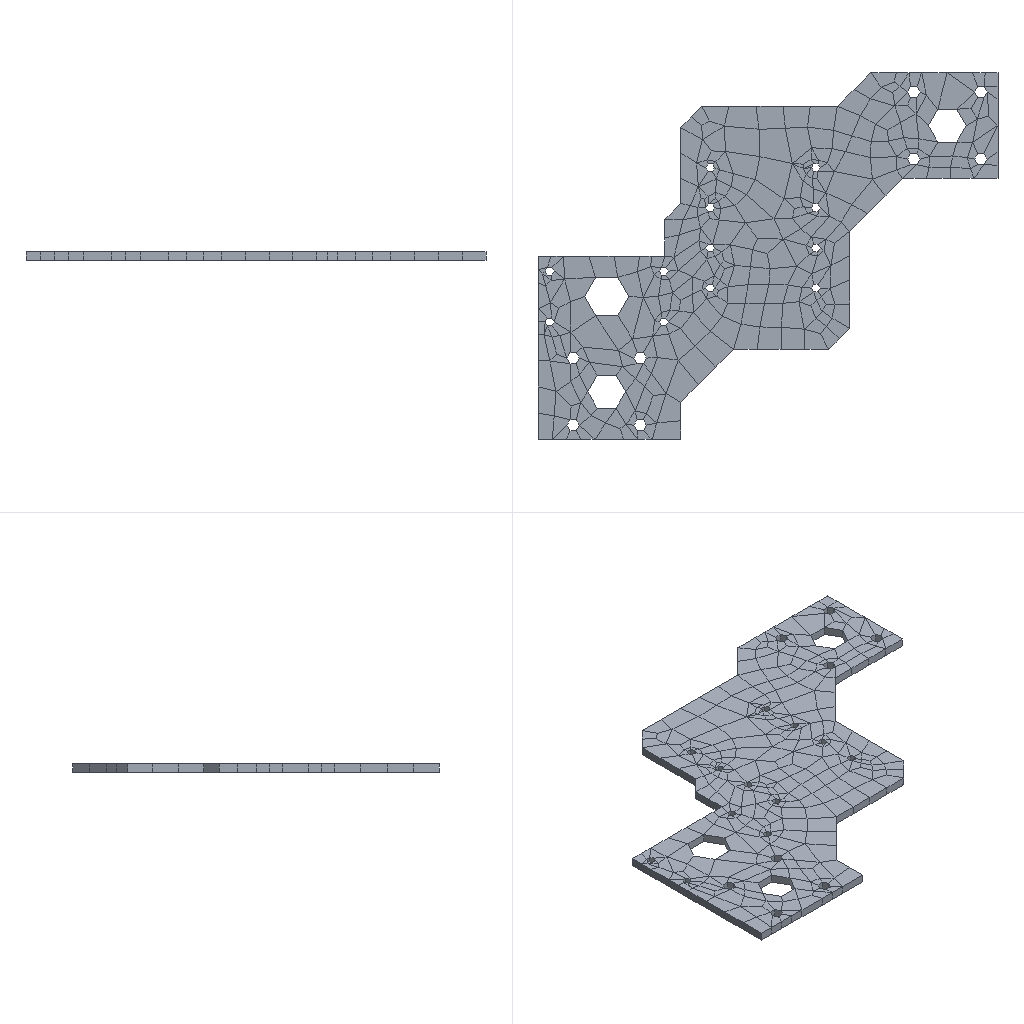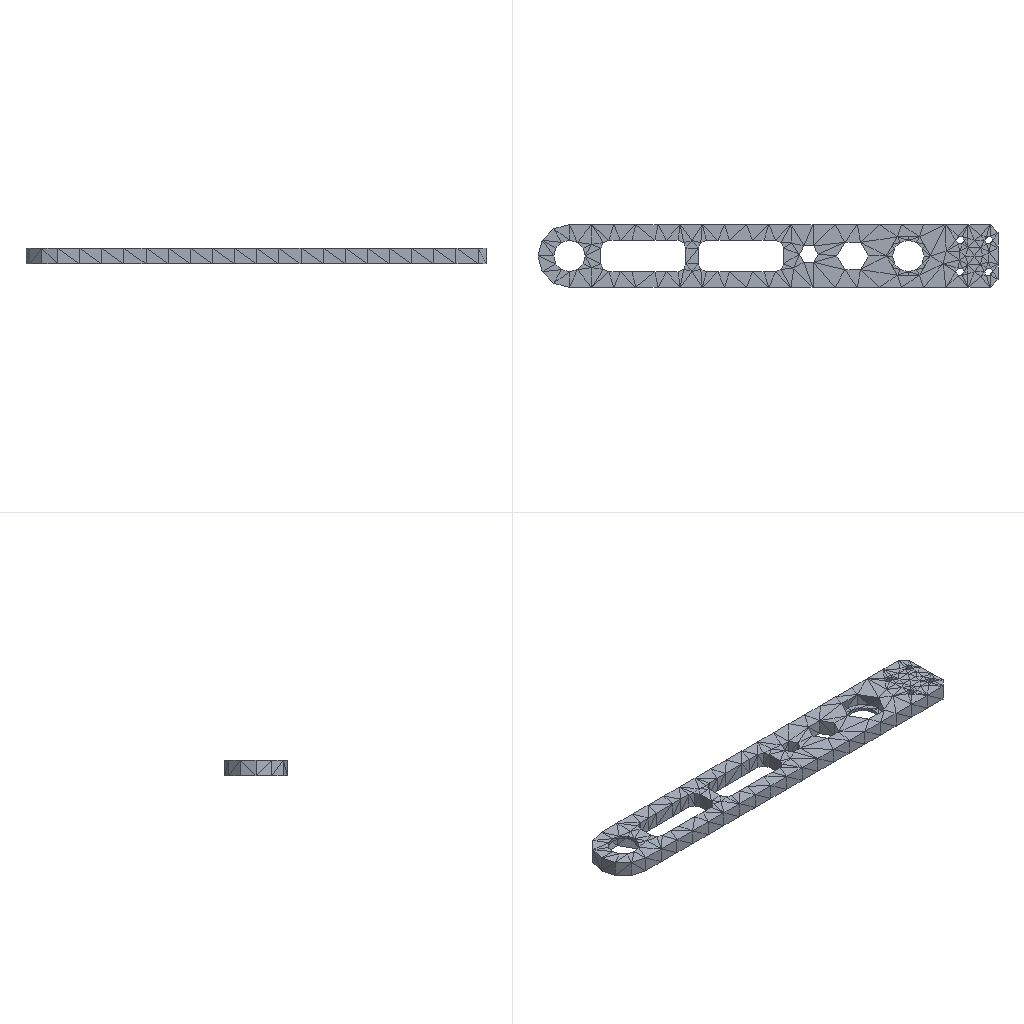Simulation study | ansys workbench
Set-up summary:
category,name,step,type,value,unit,region
solver,ansys_mapdl
solver,version,,,22.1
solver,version,,,22.1
solver,version,,,22.1
units,MPA,,stated
analysis,deck1,,static,static
load_step,requested,,,1
analysis,nlgeom,,,False
mesh,nodes,,,6576
mesh,elements,,,4228
element_type,ANSYS 187 (type 1),,solid,3574
element_type,ANSYS 174 (type 2),,contact,654
element_type,ANSYS 170 (type 3),,target,0
load,load commands in deck,,count,3
bc,support commands in deck,,count,1
named_set,_FIXEDSU,,component
analysis,deck2,,static,static
load_step,requested,,,1
analysis,nlgeom,,,False
mesh,nodes,,,2402
mesh,elements,,,1297
element_type,ANSYS 187 (type 1),,solid,1086
element_type,ANSYS 154 (type 2),,surface,211
load,load commands in deck,,count,3
bc,support commands in deck,,count,1
named_set,_FIXEDSU,,component
analysis,deck3,,static,static
load_step,requested,,,1
analysis,nlgeom,,,False
mesh,nodes,,,2920
mesh,elements,,,706
element_type,ANSYS 186 (type 1),,solid,353
element_type,ANSYS 154 (type 2),,surface,353
load,load commands in deck,,count,3
bc,support commands in deck,,count,1
named_set,_FIXEDSU,,component
material,1,,in results
material,1,,in results
material,1,,in results
check,setup vs results,,match,results also hold 0 node(s) and 1 element(s) the deck makes with ['EN']; those were not compared; 1 node(s) the solver created internally for pilot nodes (ansys-fenxi-2/轴机械结构有限元分析/111_files/dp0/SYS-1/MECH/solve.out) are in the results only
check,setup vs results,,match,211 surface effect element(s) are not in the reader's mesh and were not compared
check,setup vs results,,match,353 surface effect element(s) are not in the reader's mesh and were not compared
Results summary:
result,analysis,,,static
result,last_loadstep,,,1
result,primary field,,,displacement
result,reaction total,1,FX,0.0,N
result,reaction total,1,FY,1e-06,N
result,reaction total,1,FZ,0.0,N
result,mass,,,0.000364,"NMM: mm, ton, N, s, mV, mA, degC"
result,analysis,,,static
result,last_loadstep,,,1
result,primary field,,,displacement
result,reaction total,1,FX,-0.0,N
result,reaction total,1,FY,0.0,N
result,reaction total,1,FZ,1000.0,N
result,mass,,,0.000609,"NMM: mm, ton, N, s, mV, mA, degC"
result,analysis,,,static
result,last_loadstep,,,1
result,primary field,,,displacement
result,reaction total,1,FX,-0.0,N
result,reaction total,1,FY,-0.0,N
result,reaction total,1,FZ,5000.0,N
result,mass,,,0.00451,"NMM: mm, ton, N, s, mV, mA, degC"